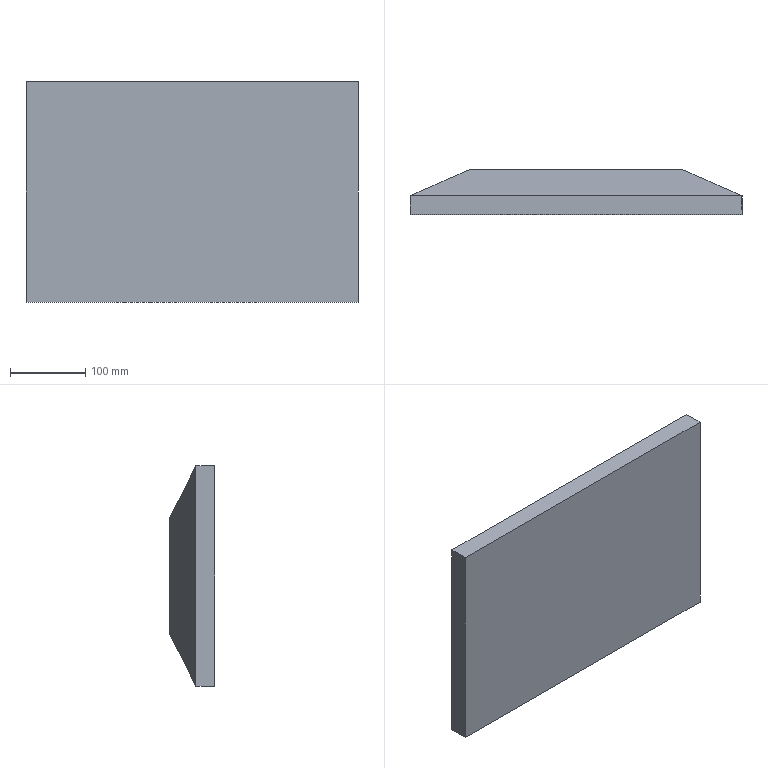Part | SolidWorks | features ICE 3, Extrusion 1 | 1 solid | 34 faces | box 440 x 60 x 292 mm | volume 6071392 mm3 | plane 18 | cylinder 16 | commonest cylinder face diameters 5 x16
STEP:
#1=CARTESIAN_POINT('',(182.5,40.,-186.));
#2=VERTEX_POINT('',#1);
#3=CARTESIAN_POINT('',(182.5,40.,-181.));
#4=VERTEX_POINT('',#3);
#5=CARTESIAN_POINT('',(182.5,40.,-183.5));
#6=DIRECTION('',(0.,1.,0.));
#7=DIRECTION('',(0.,0.,1.));
#8=AXIS2_PLACEMENT_3D('',#5,#6,#7);
#9=CIRCLE('',#8,2.5);
#10=EDGE_CURVE('',#2,#4,#9,.T.);
#11=ORIENTED_EDGE('',*,*,#10,.F.);
#12=CARTESIAN_POINT('',(182.5,60.,-186.));
#13=VERTEX_POINT('',#12);
#14=CARTESIAN_POINT('',(182.5,40.,-186.));
#15=DIRECTION('',(0.,1.,0.));
#16=VECTOR('',#15,1000.);
#17=LINE('',#14,#16);
#18=EDGE_CURVE('',#2,#13,#17,.T.);
#19=ORIENTED_EDGE('',*,*,#18,.T.);
#20=CARTESIAN_POINT('',(182.5,60.,-181.));
#21=VERTEX_POINT('',#20);
#22=CARTESIAN_POINT('',(182.5,60.,-183.5));
#23=DIRECTION('',(0.,1.,0.));
#24=DIRECTION('',(0.,0.,1.));
#25=AXIS2_PLACEMENT_3D('',#22,#23,#24);
#26=CIRCLE('',#25,2.5);
#27=EDGE_CURVE('',#13,#21,#26,.T.);
#28=ORIENTED_EDGE('',*,*,#27,.T.);
#29=CARTESIAN_POINT('',(182.5,40.,-181.));
#30=DIRECTION('',(0.,1.,0.));
#31=VECTOR('',#30,1000.);
#32=LINE('',#29,#31);
#33=EDGE_CURVE('',#4,#21,#32,.T.);
#34=ORIENTED_EDGE('',*,*,#33,.F.);
#35=EDGE_LOOP('',(#11,#19,#28,#34));
#36=FACE_OUTER_BOUND('',#35,.T.);
#37=CARTESIAN_POINT('',(182.5,40.,-183.5));
#38=DIRECTION('',(0.,1.,0.));
#39=DIRECTION('',(0.,0.,1.));
#40=AXIS2_PLACEMENT_3D('',#37,#38,#39);
#41=CYLINDRICAL_SURFACE('',#40,2.5);
#42=ADVANCED_FACE('',(#36),#41,.F.);
#43=CARTESIAN_POINT('',(170.,40.,-198.5));
#44=VERTEX_POINT('',#43);
#45=CARTESIAN_POINT('',(170.,40.,-193.5));
#46=VERTEX_POINT('',#45);
#47=CARTESIAN_POINT('',(170.,40.,-196.));
#48=DIRECTION('',(0.,1.,0.));
#49=DIRECTION('',(0.,0.,1.));
#50=AXIS2_PLACEMENT_3D('',#47,#48,#49);
#51=CIRCLE('',#50,2.5);
#52=EDGE_CURVE('',#44,#46,#51,.T.);
#53=ORIENTED_EDGE('',*,*,#52,.F.);
#54=CARTESIAN_POINT('',(170.,60.,-198.5));
#55=VERTEX_POINT('',#54);
#56=CARTESIAN_POINT('',(170.,40.,-198.5));
#57=DIRECTION('',(0.,1.,0.));
#58=VECTOR('',#57,1000.);
#59=LINE('',#56,#58);
#60=EDGE_CURVE('',#44,#55,#59,.T.);
#61=ORIENTED_EDGE('',*,*,#60,.T.);
#62=CARTESIAN_POINT('',(170.,60.,-193.5));
#63=VERTEX_POINT('',#62);
#64=CARTESIAN_POINT('',(170.,60.,-196.));
#65=DIRECTION('',(0.,1.,0.));
#66=DIRECTION('',(0.,0.,1.));
#67=AXIS2_PLACEMENT_3D('',#64,#65,#66);
#68=CIRCLE('',#67,2.5);
#69=EDGE_CURVE('',#55,#63,#68,.T.);
#70=ORIENTED_EDGE('',*,*,#69,.T.);
#71=CARTESIAN_POINT('',(170.,40.,-193.5));
#72=DIRECTION('',(0.,1.,0.));
#73=VECTOR('',#72,1000.);
#74=LINE('',#71,#73);
#75=EDGE_CURVE('',#46,#63,#74,.T.);
#76=ORIENTED_EDGE('',*,*,#75,.F.);
#77=EDGE_LOOP('',(#53,#61,#70,#76));
#78=FACE_OUTER_BOUND('',#77,.T.);
#79=CARTESIAN_POINT('',(170.,40.,-196.));
#80=DIRECTION('',(0.,1.,0.));
#81=DIRECTION('',(0.,0.,1.));
#82=AXIS2_PLACEMENT_3D('',#79,#80,#81);
#83=CYLINDRICAL_SURFACE('',#82,2.5);
#84=ADVANCED_FACE('',(#78),#83,.F.);
#85=CARTESIAN_POINT('',(182.5,40.,-111.));
#86=VERTEX_POINT('',#85);
#87=CARTESIAN_POINT('',(182.5,40.,-106.));
#88=VERTEX_POINT('',#87);
#89=CARTESIAN_POINT('',(182.5,40.,-108.5));
#90=DIRECTION('',(0.,1.,0.));
#91=DIRECTION('',(0.,0.,1.));
#92=AXIS2_PLACEMENT_3D('',#89,#90,#91);
#93=CIRCLE('',#92,2.5);
#94=EDGE_CURVE('',#86,#88,#93,.T.);
#95=ORIENTED_EDGE('',*,*,#94,.F.);
#96=CARTESIAN_POINT('',(182.5,60.,-111.));
#97=VERTEX_POINT('',#96);
#98=CARTESIAN_POINT('',(182.5,40.,-111.));
#99=DIRECTION('',(0.,1.,0.));
#100=VECTOR('',#99,1000.);
#101=LINE('',#98,#100);
#102=EDGE_CURVE('',#86,#97,#101,.T.);
#103=ORIENTED_EDGE('',*,*,#102,.T.);
#104=CARTESIAN_POINT('',(182.5,60.,-106.));
#105=VERTEX_POINT('',#104);
#106=CARTESIAN_POINT('',(182.5,60.,-108.5));
#107=DIRECTION('',(0.,1.,0.));
#108=DIRECTION('',(0.,0.,1.));
#109=AXIS2_PLACEMENT_3D('',#106,#107,#108);
#110=CIRCLE('',#109,2.5);
#111=EDGE_CURVE('',#97,#105,#110,.T.);
#112=ORIENTED_EDGE('',*,*,#111,.T.);
#113=CARTESIAN_POINT('',(182.5,40.,-106.));
#114=DIRECTION('',(0.,1.,0.));
#115=VECTOR('',#114,1000.);
#116=LINE('',#113,#115);
#117=EDGE_CURVE('',#88,#105,#116,.T.);
#118=ORIENTED_EDGE('',*,*,#117,.F.);
#119=EDGE_LOOP('',(#95,#103,#112,#118));
#120=FACE_OUTER_BOUND('',#119,.T.);
#121=CARTESIAN_POINT('',(182.5,40.,-108.5));
#122=DIRECTION('',(0.,1.,0.));
#123=DIRECTION('',(0.,0.,1.));
#124=AXIS2_PLACEMENT_3D('',#121,#122,#123);
#125=CYLINDRICAL_SURFACE('',#124,2.5);
#126=ADVANCED_FACE('',(#120),#125,.F.);
#127=CARTESIAN_POINT('',(170.,40.,-98.5));
#128=VERTEX_POINT('',#127);
#129=CARTESIAN_POINT('',(170.,40.,-93.5));
#130=VERTEX_POINT('',#129);
#131=CARTESIAN_POINT('',(170.,40.,-96.));
#132=DIRECTION('',(0.,1.,0.));
#133=DIRECTION('',(0.,0.,1.));
#134=AXIS2_PLACEMENT_3D('',#131,#132,#133);
#135=CIRCLE('',#134,2.5);
#136=EDGE_CURVE('',#128,#130,#135,.T.);
#137=ORIENTED_EDGE('',*,*,#136,.F.);
#138=CARTESIAN_POINT('',(170.,60.,-98.5));
#139=VERTEX_POINT('',#138);
#140=CARTESIAN_POINT('',(170.,40.,-98.5));
#141=DIRECTION('',(0.,1.,0.));
#142=VECTOR('',#141,1000.);
#143=LINE('',#140,#142);
#144=EDGE_CURVE('',#128,#139,#143,.T.);
#145=ORIENTED_EDGE('',*,*,#144,.T.);
#146=CARTESIAN_POINT('',(170.,60.,-93.5));
#147=VERTEX_POINT('',#146);
#148=CARTESIAN_POINT('',(170.,60.,-96.));
#149=DIRECTION('',(0.,1.,0.));
#150=DIRECTION('',(0.,0.,1.));
#151=AXIS2_PLACEMENT_3D('',#148,#149,#150);
#152=CIRCLE('',#151,2.5);
#153=EDGE_CURVE('',#139,#147,#152,.T.);
#154=ORIENTED_EDGE('',*,*,#153,.T.);
#155=CARTESIAN_POINT('',(170.,40.,-93.5));
#156=DIRECTION('',(0.,1.,0.));
#157=VECTOR('',#156,1000.);
#158=LINE('',#155,#157);
#159=EDGE_CURVE('',#130,#147,#158,.T.);
#160=ORIENTED_EDGE('',*,*,#159,.F.);
#161=EDGE_LOOP('',(#137,#145,#154,#160));
#162=FACE_OUTER_BOUND('',#161,.T.);
#163=CARTESIAN_POINT('',(170.,40.,-96.));
#164=DIRECTION('',(0.,1.,0.));
#165=DIRECTION('',(0.,0.,1.));
#166=AXIS2_PLACEMENT_3D('',#163,#164,#165);
#167=CYLINDRICAL_SURFACE('',#166,2.5);
#168=ADVANCED_FACE('',(#162),#167,.F.);
#169=CARTESIAN_POINT('',(257.5,40.,-111.));
#170=VERTEX_POINT('',#169);
#171=CARTESIAN_POINT('',(257.5,40.,-106.));
#172=VERTEX_POINT('',#171);
#173=CARTESIAN_POINT('',(257.5,40.,-108.5));
#174=DIRECTION('',(0.,1.,0.));
#175=DIRECTION('',(0.,0.,1.));
#176=AXIS2_PLACEMENT_3D('',#173,#174,#175);
#177=CIRCLE('',#176,2.5);
#178=EDGE_CURVE('',#170,#172,#177,.T.);
#179=ORIENTED_EDGE('',*,*,#178,.F.);
#180=CARTESIAN_POINT('',(257.5,60.,-111.));
#181=VERTEX_POINT('',#180);
#182=CARTESIAN_POINT('',(257.5,40.,-111.));
#183=DIRECTION('',(0.,1.,0.));
#184=VECTOR('',#183,1000.);
#185=LINE('',#182,#184);
#186=EDGE_CURVE('',#170,#181,#185,.T.);
#187=ORIENTED_EDGE('',*,*,#186,.T.);
#188=CARTESIAN_POINT('',(257.5,60.,-106.));
#189=VERTEX_POINT('',#188);
#190=CARTESIAN_POINT('',(257.5,60.,-108.5));
#191=DIRECTION('',(0.,1.,0.));
#192=DIRECTION('',(0.,0.,1.));
#193=AXIS2_PLACEMENT_3D('',#190,#191,#192);
#194=CIRCLE('',#193,2.5);
#195=EDGE_CURVE('',#181,#189,#194,.T.);
#196=ORIENTED_EDGE('',*,*,#195,.T.);
#197=CARTESIAN_POINT('',(257.5,40.,-106.));
#198=DIRECTION('',(0.,1.,0.));
#199=VECTOR('',#198,1000.);
#200=LINE('',#197,#199);
#201=EDGE_CURVE('',#172,#189,#200,.T.);
#202=ORIENTED_EDGE('',*,*,#201,.F.);
#203=EDGE_LOOP('',(#179,#187,#196,#202));
#204=FACE_OUTER_BOUND('',#203,.T.);
#205=CARTESIAN_POINT('',(257.5,40.,-108.5));
#206=DIRECTION('',(0.,1.,0.));
#207=DIRECTION('',(0.,0.,1.));
#208=AXIS2_PLACEMENT_3D('',#205,#206,#207);
#209=CYLINDRICAL_SURFACE('',#208,2.5);
#210=ADVANCED_FACE('',(#204),#209,.F.);
#211=CARTESIAN_POINT('',(270.,40.,-98.5));
#212=VERTEX_POINT('',#211);
#213=CARTESIAN_POINT('',(270.,40.,-93.5));
#214=VERTEX_POINT('',#213);
#215=CARTESIAN_POINT('',(270.,40.,-96.));
#216=DIRECTION('',(0.,1.,0.));
#217=DIRECTION('',(0.,0.,1.));
#218=AXIS2_PLACEMENT_3D('',#215,#216,#217);
#219=CIRCLE('',#218,2.5);
#220=EDGE_CURVE('',#212,#214,#219,.T.);
#221=ORIENTED_EDGE('',*,*,#220,.F.);
#222=CARTESIAN_POINT('',(270.,60.,-98.5));
#223=VERTEX_POINT('',#222);
#224=CARTESIAN_POINT('',(270.,40.,-98.5));
#225=DIRECTION('',(0.,1.,0.));
#226=VECTOR('',#225,1000.);
#227=LINE('',#224,#226);
#228=EDGE_CURVE('',#212,#223,#227,.T.);
#229=ORIENTED_EDGE('',*,*,#228,.T.);
#230=CARTESIAN_POINT('',(270.,60.,-93.5));
#231=VERTEX_POINT('',#230);
#232=CARTESIAN_POINT('',(270.,60.,-96.));
#233=DIRECTION('',(0.,1.,0.));
#234=DIRECTION('',(0.,0.,1.));
#235=AXIS2_PLACEMENT_3D('',#232,#233,#234);
#236=CIRCLE('',#235,2.5);
#237=EDGE_CURVE('',#223,#231,#236,.T.);
#238=ORIENTED_EDGE('',*,*,#237,.T.);
#239=CARTESIAN_POINT('',(270.,40.,-93.5));
#240=DIRECTION('',(0.,1.,0.));
#241=VECTOR('',#240,1000.);
#242=LINE('',#239,#241);
#243=EDGE_CURVE('',#214,#231,#242,.T.);
#244=ORIENTED_EDGE('',*,*,#243,.F.);
#245=EDGE_LOOP('',(#221,#229,#238,#244));
#246=FACE_OUTER_BOUND('',#245,.T.);
#247=CARTESIAN_POINT('',(270.,40.,-96.));
#248=DIRECTION('',(0.,1.,0.));
#249=DIRECTION('',(0.,0.,1.));
#250=AXIS2_PLACEMENT_3D('',#247,#248,#249);
#251=CYLINDRICAL_SURFACE('',#250,2.5);
#252=ADVANCED_FACE('',(#246),#251,.F.);
#253=CARTESIAN_POINT('',(257.5,40.,-186.));
#254=VERTEX_POINT('',#253);
#255=CARTESIAN_POINT('',(257.5,40.,-181.));
#256=VERTEX_POINT('',#255);
#257=CARTESIAN_POINT('',(257.5,40.,-183.5));
#258=DIRECTION('',(0.,1.,0.));
#259=DIRECTION('',(0.,0.,1.));
#260=AXIS2_PLACEMENT_3D('',#257,#258,#259);
#261=CIRCLE('',#260,2.5);
#262=EDGE_CURVE('',#254,#256,#261,.T.);
#263=ORIENTED_EDGE('',*,*,#262,.F.);
#264=CARTESIAN_POINT('',(257.5,60.,-186.));
#265=VERTEX_POINT('',#264);
#266=CARTESIAN_POINT('',(257.5,40.,-186.));
#267=DIRECTION('',(0.,1.,0.));
#268=VECTOR('',#267,1000.);
#269=LINE('',#266,#268);
#270=EDGE_CURVE('',#254,#265,#269,.T.);
#271=ORIENTED_EDGE('',*,*,#270,.T.);
#272=CARTESIAN_POINT('',(257.5,60.,-181.));
#273=VERTEX_POINT('',#272);
#274=CARTESIAN_POINT('',(257.5,60.,-183.5));
#275=DIRECTION('',(0.,1.,0.));
#276=DIRECTION('',(0.,0.,1.));
#277=AXIS2_PLACEMENT_3D('',#274,#275,#276);
#278=CIRCLE('',#277,2.5);
#279=EDGE_CURVE('',#265,#273,#278,.T.);
#280=ORIENTED_EDGE('',*,*,#279,.T.);
#281=CARTESIAN_POINT('',(257.5,40.,-181.));
#282=DIRECTION('',(0.,1.,0.));
#283=VECTOR('',#282,1000.);
#284=LINE('',#281,#283);
#285=EDGE_CURVE('',#256,#273,#284,.T.);
#286=ORIENTED_EDGE('',*,*,#285,.F.);
#287=EDGE_LOOP('',(#263,#271,#280,#286));
#288=FACE_OUTER_BOUND('',#287,.T.);
#289=CARTESIAN_POINT('',(257.5,40.,-183.5));
#290=DIRECTION('',(0.,1.,0.));
#291=DIRECTION('',(0.,0.,1.));
#292=AXIS2_PLACEMENT_3D('',#289,#290,#291);
#293=CYLINDRICAL_SURFACE('',#292,2.5);
#294=ADVANCED_FACE('',(#288),#293,.F.);
#295=CARTESIAN_POINT('',(270.,40.,-198.5));
#296=VERTEX_POINT('',#295);
#297=CARTESIAN_POINT('',(270.,40.,-193.5));
#298=VERTEX_POINT('',#297);
#299=CARTESIAN_POINT('',(270.,40.,-196.));
#300=DIRECTION('',(0.,1.,0.));
#301=DIRECTION('',(0.,0.,1.));
#302=AXIS2_PLACEMENT_3D('',#299,#300,#301);
#303=CIRCLE('',#302,2.5);
#304=EDGE_CURVE('',#296,#298,#303,.T.);
#305=ORIENTED_EDGE('',*,*,#304,.F.);
#306=CARTESIAN_POINT('',(270.,60.,-198.5));
#307=VERTEX_POINT('',#306);
#308=CARTESIAN_POINT('',(270.,40.,-198.5));
#309=DIRECTION('',(0.,1.,0.));
#310=VECTOR('',#309,1000.);
#311=LINE('',#308,#310);
#312=EDGE_CURVE('',#296,#307,#311,.T.);
#313=ORIENTED_EDGE('',*,*,#312,.T.);
#314=CARTESIAN_POINT('',(270.,60.,-193.5));
#315=VERTEX_POINT('',#314);
#316=CARTESIAN_POINT('',(270.,60.,-196.));
#317=DIRECTION('',(0.,1.,0.));
#318=DIRECTION('',(0.,0.,1.));
#319=AXIS2_PLACEMENT_3D('',#316,#317,#318);
#320=CIRCLE('',#319,2.5);
#321=EDGE_CURVE('',#307,#315,#320,.T.);
#322=ORIENTED_EDGE('',*,*,#321,.T.);
#323=CARTESIAN_POINT('',(270.,40.,-193.5));
#324=DIRECTION('',(0.,1.,0.));
#325=VECTOR('',#324,1000.);
#326=LINE('',#323,#325);
#327=EDGE_CURVE('',#298,#315,#326,.T.);
#328=ORIENTED_EDGE('',*,*,#327,.F.);
#329=EDGE_LOOP('',(#305,#313,#322,#328));
#330=FACE_OUTER_BOUND('',#329,.T.);
#331=CARTESIAN_POINT('',(270.,40.,-196.));
#332=DIRECTION('',(0.,1.,0.));
#333=DIRECTION('',(0.,0.,1.));
#334=AXIS2_PLACEMENT_3D('',#331,#332,#333);
#335=CYLINDRICAL_SURFACE('',#334,2.5);
#336=ADVANCED_FACE('',(#330),#335,.F.);
#337=CARTESIAN_POINT('',(0.,25.,0.));
#338=VERTEX_POINT('',#337);
#339=CARTESIAN_POINT('',(0.,0.,0.));
#340=VERTEX_POINT('',#339);
#341=CARTESIAN_POINT('',(0.,60.,0.));
#342=DIRECTION('',(0.,-1.,0.));
#343=VECTOR('',#342,1000.);
#344=LINE('',#341,#343);
#345=EDGE_CURVE('',#338,#340,#344,.T.);
#346=ORIENTED_EDGE('',*,*,#345,.F.);
#347=CARTESIAN_POINT('',(0.,25.,-292.));
#348=VERTEX_POINT('',#347);
#349=CARTESIAN_POINT('',(0.,25.,87.));
#350=DIRECTION('',(0.,0.,-1.));
#351=VECTOR('',#350,1000.);
#352=LINE('',#349,#351);
#353=EDGE_CURVE('',#338,#348,#352,.T.);
#354=ORIENTED_EDGE('',*,*,#353,.T.);
#355=CARTESIAN_POINT('',(0.,0.,-292.));
#356=VERTEX_POINT('',#355);
#357=CARTESIAN_POINT('',(0.,60.,-292.));
#358=DIRECTION('',(0.,-1.,0.));
#359=VECTOR('',#358,1000.);
#360=LINE('',#357,#359);
#361=EDGE_CURVE('',#348,#356,#360,.T.);
#362=ORIENTED_EDGE('',*,*,#361,.T.);
#363=CARTESIAN_POINT('',(0.,0.,0.));
#364=DIRECTION('',(0.,0.,1.));
#365=VECTOR('',#364,1000.);
#366=LINE('',#363,#365);
#367=EDGE_CURVE('',#356,#340,#366,.T.);
#368=ORIENTED_EDGE('',*,*,#367,.T.);
#369=EDGE_LOOP('',(#346,#354,#362,#368));
#370=FACE_OUTER_BOUND('',#369,.T.);
#371=CARTESIAN_POINT('',(0.,60.,0.));
#372=DIRECTION('',(1.,0.,0.));
#373=DIRECTION('',(0.,0.,-1.));
#374=AXIS2_PLACEMENT_3D('',#371,#372,#373);
#375=PLANE('',#374);
#376=ADVANCED_FACE('',(#370),#375,.F.);
#377=CARTESIAN_POINT('',(440.,25.,0.));
#378=VERTEX_POINT('',#377);
#379=CARTESIAN_POINT('',(440.,0.,0.));
#380=VERTEX_POINT('',#379);
#381=CARTESIAN_POINT('',(440.,60.,0.));
#382=DIRECTION('',(0.,-1.,0.));
#383=VECTOR('',#382,1000.);
#384=LINE('',#381,#383);
#385=EDGE_CURVE('',#378,#380,#384,.T.);
#386=ORIENTED_EDGE('',*,*,#385,.F.);
#387=CARTESIAN_POINT('',(467.,25.,0.));
#388=DIRECTION('',(-1.,0.,0.));
#389=VECTOR('',#388,1000.);
#390=LINE('',#387,#389);
#391=EDGE_CURVE('',#378,#338,#390,.T.);
#392=ORIENTED_EDGE('',*,*,#391,.T.);
#393=ORIENTED_EDGE('',*,*,#345,.T.);
#394=CARTESIAN_POINT('',(0.,0.,0.));
#395=DIRECTION('',(1.,0.,0.));
#396=VECTOR('',#395,1000.);
#397=LINE('',#394,#396);
#398=EDGE_CURVE('',#340,#380,#397,.T.);
#399=ORIENTED_EDGE('',*,*,#398,.T.);
#400=EDGE_LOOP('',(#386,#392,#393,#399));
#401=FACE_OUTER_BOUND('',#400,.T.);
#402=CARTESIAN_POINT('',(0.,60.,0.));
#403=DIRECTION('',(0.,0.,-1.));
#404=DIRECTION('',(-1.,0.,0.));
#405=AXIS2_PLACEMENT_3D('',#402,#403,#404);
#406=PLANE('',#405);
#407=ADVANCED_FACE('',(#401),#406,.F.);
#408=CARTESIAN_POINT('',(440.,25.,-292.));
#409=VERTEX_POINT('',#408);
#410=CARTESIAN_POINT('',(440.,0.,-292.));
#411=VERTEX_POINT('',#410);
#412=CARTESIAN_POINT('',(440.,60.,-292.));
#413=DIRECTION('',(0.,-1.,0.));
#414=VECTOR('',#413,1000.);
#415=LINE('',#412,#414);
#416=EDGE_CURVE('',#409,#411,#415,.T.);
#417=ORIENTED_EDGE('',*,*,#416,.F.);
#418=CARTESIAN_POINT('',(440.,25.,87.));
#419=DIRECTION('',(0.,0.,-1.));
#420=VECTOR('',#419,1000.);
#421=LINE('',#418,#420);
#422=EDGE_CURVE('',#378,#409,#421,.T.);
#423=ORIENTED_EDGE('',*,*,#422,.F.);
#424=ORIENTED_EDGE('',*,*,#385,.T.);
#425=CARTESIAN_POINT('',(440.,0.,0.));
#426=DIRECTION('',(0.,0.,-1.));
#427=VECTOR('',#426,1000.);
#428=LINE('',#425,#427);
#429=EDGE_CURVE('',#380,#411,#428,.T.);
#430=ORIENTED_EDGE('',*,*,#429,.T.);
#431=EDGE_LOOP('',(#417,#423,#424,#430));
#432=FACE_OUTER_BOUND('',#431,.T.);
#433=CARTESIAN_POINT('',(440.,60.,0.));
#434=DIRECTION('',(-1.,0.,0.));
#435=DIRECTION('',(0.,0.,1.));
#436=AXIS2_PLACEMENT_3D('',#433,#434,#435);
#437=PLANE('',#436);
#438=ADVANCED_FACE('',(#432),#437,.F.);
#439=ORIENTED_EDGE('',*,*,#361,.F.);
#440=CARTESIAN_POINT('',(467.,25.,-292.));
#441=DIRECTION('',(-1.,0.,0.));
#442=VECTOR('',#441,1000.);
#443=LINE('',#440,#442);
#444=EDGE_CURVE('',#409,#348,#443,.T.);
#445=ORIENTED_EDGE('',*,*,#444,.F.);
#446=ORIENTED_EDGE('',*,*,#416,.T.);
#447=CARTESIAN_POINT('',(0.,0.,-292.));
#448=DIRECTION('',(-1.,0.,0.));
#449=VECTOR('',#448,1000.);
#450=LINE('',#447,#449);
#451=EDGE_CURVE('',#411,#356,#450,.T.);
#452=ORIENTED_EDGE('',*,*,#451,.T.);
#453=EDGE_LOOP('',(#439,#445,#446,#452));
#454=FACE_OUTER_BOUND('',#453,.T.);
#455=CARTESIAN_POINT('',(0.,60.,-292.));
#456=DIRECTION('',(0.,0.,1.));
#457=DIRECTION('',(1.,0.,0.));
#458=AXIS2_PLACEMENT_3D('',#455,#456,#457);
#459=PLANE('',#458);
#460=ADVANCED_FACE('',(#454),#459,.F.);
#461=CARTESIAN_POINT('',(182.5,60.,-183.5));
#462=DIRECTION('',(0.,1.,0.));
#463=DIRECTION('',(0.,0.,1.));
#464=AXIS2_PLACEMENT_3D('',#461,#462,#463);
#465=CIRCLE('',#464,2.5);
#466=EDGE_CURVE('',#21,#13,#465,.T.);
#467=ORIENTED_EDGE('',*,*,#466,.F.);
#468=ORIENTED_EDGE('',*,*,#27,.F.);
#469=EDGE_LOOP('',(#467,#468));
#470=FACE_BOUND('',#469,.T.);
#471=CARTESIAN_POINT('',(170.,60.,-196.));
#472=DIRECTION('',(0.,1.,0.));
#473=DIRECTION('',(0.,0.,1.));
#474=AXIS2_PLACEMENT_3D('',#471,#472,#473);
#475=CIRCLE('',#474,2.5);
#476=EDGE_CURVE('',#63,#55,#475,.T.);
#477=ORIENTED_EDGE('',*,*,#476,.F.);
#478=ORIENTED_EDGE('',*,*,#69,.F.);
#479=EDGE_LOOP('',(#477,#478));
#480=FACE_BOUND('',#479,.T.);
#481=CARTESIAN_POINT('',(182.5,60.,-108.5));
#482=DIRECTION('',(0.,1.,0.));
#483=DIRECTION('',(0.,0.,1.));
#484=AXIS2_PLACEMENT_3D('',#481,#482,#483);
#485=CIRCLE('',#484,2.5);
#486=EDGE_CURVE('',#105,#97,#485,.T.);
#487=ORIENTED_EDGE('',*,*,#486,.F.);
#488=ORIENTED_EDGE('',*,*,#111,.F.);
#489=EDGE_LOOP('',(#487,#488));
#490=FACE_BOUND('',#489,.T.);
#491=CARTESIAN_POINT('',(170.,60.,-96.));
#492=DIRECTION('',(0.,1.,0.));
#493=DIRECTION('',(0.,0.,1.));
#494=AXIS2_PLACEMENT_3D('',#491,#492,#493);
#495=CIRCLE('',#494,2.5);
#496=EDGE_CURVE('',#147,#139,#495,.T.);
#497=ORIENTED_EDGE('',*,*,#496,.F.);
#498=ORIENTED_EDGE('',*,*,#153,.F.);
#499=EDGE_LOOP('',(#497,#498));
#500=FACE_BOUND('',#499,.T.);
#501=CARTESIAN_POINT('',(257.5,60.,-108.5));
#502=DIRECTION('',(0.,1.,0.));
#503=DIRECTION('',(0.,0.,1.));
#504=AXIS2_PLACEMENT_3D('',#501,#502,#503);
#505=CIRCLE('',#504,2.5);
#506=EDGE_CURVE('',#189,#181,#505,.T.);
#507=ORIENTED_EDGE('',*,*,#506,.F.);
#508=ORIENTED_EDGE('',*,*,#195,.F.);
#509=EDGE_LOOP('',(#507,#508));
#510=FACE_BOUND('',#509,.T.);
#511=CARTESIAN_POINT('',(270.,60.,-96.));
#512=DIRECTION('',(0.,1.,0.));
#513=DIRECTION('',(0.,0.,1.));
#514=AXIS2_PLACEMENT_3D('',#511,#512,#513);
#515=CIRCLE('',#514,2.5);
#516=EDGE_CURVE('',#231,#223,#515,.T.);
#517=ORIENTED_EDGE('',*,*,#516,.F.);
#518=ORIENTED_EDGE('',*,*,#237,.F.);
#519=EDGE_LOOP('',(#517,#518));
#520=FACE_BOUND('',#519,.T.);
#521=CARTESIAN_POINT('',(257.5,60.,-183.5));
#522=DIRECTION('',(0.,1.,0.));
#523=DIRECTION('',(0.,0.,1.));
#524=AXIS2_PLACEMENT_3D('',#521,#522,#523);
#525=CIRCLE('',#524,2.5);
#526=EDGE_CURVE('',#273,#265,#525,.T.);
#527=ORIENTED_EDGE('',*,*,#526,.F.);
#528=ORIENTED_EDGE('',*,*,#279,.F.);
#529=EDGE_LOOP('',(#527,#528));
#530=FACE_BOUND('',#529,.T.);
#531=CARTESIAN_POINT('',(270.,60.,-196.));
#532=DIRECTION('',(0.,1.,0.));
#533=DIRECTION('',(0.,0.,1.));
#534=AXIS2_PLACEMENT_3D('',#531,#532,#533);
#535=CIRCLE('',#534,2.5);
#536=EDGE_CURVE('',#315,#307,#535,.T.);
#537=ORIENTED_EDGE('',*,*,#536,.F.);
#538=ORIENTED_EDGE('',*,*,#321,.F.);
#539=EDGE_LOOP('',(#537,#538));
#540=FACE_BOUND('',#539,.T.);
#541=CARTESIAN_POINT('',(80.,60.,-222.));
#542=VERTEX_POINT('',#541);
#543=CARTESIAN_POINT('',(80.,60.,-70.));
#544=VERTEX_POINT('',#543);
#545=CARTESIAN_POINT('',(80.,60.,-292.));
#546=DIRECTION('',(0.,0.,1.));
#547=VECTOR('',#546,1000.);
#548=LINE('',#545,#547);
#549=EDGE_CURVE('',#542,#544,#548,.T.);
#550=ORIENTED_EDGE('',*,*,#549,.T.);
#551=CARTESIAN_POINT('',(360.,60.,-70.));
#552=VERTEX_POINT('',#551);
#553=CARTESIAN_POINT('',(467.,60.,-70.));
#554=DIRECTION('',(-1.,0.,0.));
#555=VECTOR('',#554,1000.);
#556=LINE('',#553,#555);
#557=EDGE_CURVE('',#552,#544,#556,.T.);
#558=ORIENTED_EDGE('',*,*,#557,.F.);
#559=CARTESIAN_POINT('',(360.,60.,-222.));
#560=VERTEX_POINT('',#559);
#561=CARTESIAN_POINT('',(360.,60.,-292.));
#562=DIRECTION('',(0.,0.,-1.));
#563=VECTOR('',#562,1000.);
#564=LINE('',#561,#563);
#565=EDGE_CURVE('',#552,#560,#564,.T.);
#566=ORIENTED_EDGE('',*,*,#565,.T.);
#567=CARTESIAN_POINT('',(467.,60.,-222.));
#568=DIRECTION('',(-1.,0.,0.));
#569=VECTOR('',#568,1000.);
#570=LINE('',#567,#569);
#571=EDGE_CURVE('',#560,#542,#570,.T.);
#572=ORIENTED_EDGE('',*,*,#571,.T.);
#573=EDGE_LOOP('',(#550,#558,#566,#572));
#574=FACE_OUTER_BOUND('',#573,.T.);
#575=CARTESIAN_POINT('',(0.,60.,-292.));
#576=DIRECTION('',(0.,-1.,0.));
#577=DIRECTION('',(0.,0.,-1.));
#578=AXIS2_PLACEMENT_3D('',#575,#576,#577);
#579=PLANE('',#578);
#580=ADVANCED_FACE('',(#470,#480,#490,#500,#510,#520,#530,#540,#574),#579,.F.);
#581=ORIENTED_EDGE('',*,*,#367,.F.);
#582=ORIENTED_EDGE('',*,*,#451,.F.);
#583=ORIENTED_EDGE('',*,*,#429,.F.);
#584=ORIENTED_EDGE('',*,*,#398,.F.);
#585=EDGE_LOOP('',(#581,#582,#583,#584));
#586=FACE_OUTER_BOUND('',#585,.T.);
#587=CARTESIAN_POINT('',(0.,0.,-292.));
#588=DIRECTION('',(0.,-1.,0.));
#589=DIRECTION('',(0.,0.,-1.));
#590=AXIS2_PLACEMENT_3D('',#587,#588,#589);
#591=PLANE('',#590);
#592=ADVANCED_FACE('',(#586),#591,.T.);
#593=ORIENTED_EDGE('',*,*,#565,.F.);
#594=CARTESIAN_POINT('',(430.196,29.289,-8.579));
#595=DIRECTION('',(0.7148,-0.3127,0.6255));
#596=VECTOR('',#595,1000.);
#597=LINE('',#594,#596);
#598=EDGE_CURVE('',#552,#378,#597,.T.);
#599=ORIENTED_EDGE('',*,*,#598,.T.);
#600=ORIENTED_EDGE('',*,*,#422,.T.);
#601=CARTESIAN_POINT('',(221.844,120.443,-101.114));
#602=DIRECTION('',(-0.7148,0.3127,0.6255));
#603=VECTOR('',#602,1000.);
#604=LINE('',#601,#603);
#605=EDGE_CURVE('',#409,#560,#604,.T.);
#606=ORIENTED_EDGE('',*,*,#605,.T.);
#607=EDGE_LOOP('',(#593,#599,#600,#606));
#608=FACE_OUTER_BOUND('',#607,.T.);
#609=CARTESIAN_POINT('',(360.,60.,87.));
#610=DIRECTION('',(-0.4008,-0.9162,0.));
#611=DIRECTION('',(0.9162,-0.4008,0.));
#612=AXIS2_PLACEMENT_3D('',#609,#610,#611);
#613=PLANE('',#612);
#614=ADVANCED_FACE('',(#608),#613,.F.);
#615=ORIENTED_EDGE('',*,*,#353,.F.);
#616=CARTESIAN_POINT('',(9.804,29.289,-8.579));
#617=DIRECTION('',(0.7148,0.3127,-0.6255));
#618=VECTOR('',#617,1000.);
#619=LINE('',#616,#618);
#620=EDGE_CURVE('',#338,#544,#619,.T.);
#621=ORIENTED_EDGE('',*,*,#620,.T.);
#622=ORIENTED_EDGE('',*,*,#549,.F.);
#623=CARTESIAN_POINT('',(218.156,120.443,-101.114));
#624=DIRECTION('',(-0.7148,-0.3127,-0.6255));
#625=VECTOR('',#624,1000.);
#626=LINE('',#623,#625);
#627=EDGE_CURVE('',#542,#348,#626,.T.);
#628=ORIENTED_EDGE('',*,*,#627,.T.);
#629=EDGE_LOOP('',(#615,#621,#622,#628));
#630=FACE_OUTER_BOUND('',#629,.T.);
#631=CARTESIAN_POINT('',(80.,60.,87.));
#632=DIRECTION('',(0.4008,-0.9162,0.));
#633=DIRECTION('',(0.9162,0.4008,0.));
#634=AXIS2_PLACEMENT_3D('',#631,#632,#633);
#635=PLANE('',#634);
#636=ADVANCED_FACE('',(#630),#635,.F.);
#637=ORIENTED_EDGE('',*,*,#444,.T.);
#638=ORIENTED_EDGE('',*,*,#627,.F.);
#639=ORIENTED_EDGE('',*,*,#571,.F.);
#640=ORIENTED_EDGE('',*,*,#605,.F.);
#641=EDGE_LOOP('',(#637,#638,#639,#640));
#642=FACE_OUTER_BOUND('',#641,.T.);
#643=CARTESIAN_POINT('',(467.,60.,-222.));
#644=DIRECTION('',(0.,-0.8944,0.4472));
#645=DIRECTION('',(0.,-0.4472,-0.8944));
#646=AXIS2_PLACEMENT_3D('',#643,#644,#645);
#647=PLANE('',#646);
#648=ADVANCED_FACE('',(#642),#647,.F.);
#649=ORIENTED_EDGE('',*,*,#557,.T.);
#650=ORIENTED_EDGE('',*,*,#620,.F.);
#651=ORIENTED_EDGE('',*,*,#391,.F.);
#652=ORIENTED_EDGE('',*,*,#598,.F.);
#653=EDGE_LOOP('',(#649,#650,#651,#652));
#654=FACE_OUTER_BOUND('',#653,.T.);
#655=CARTESIAN_POINT('',(467.,60.,-70.));
#656=DIRECTION('',(0.,-0.8944,-0.4472));
#657=DIRECTION('',(0.,0.4472,-0.8944));
#658=AXIS2_PLACEMENT_3D('',#655,#656,#657);
#659=PLANE('',#658);
#660=ADVANCED_FACE('',(#654),#659,.F.);
#661=ORIENTED_EDGE('',*,*,#312,.F.);
#662=CARTESIAN_POINT('',(270.,40.,-196.));
#663=DIRECTION('',(0.,1.,0.));
#664=DIRECTION('',(0.,0.,1.));
#665=AXIS2_PLACEMENT_3D('',#662,#663,#664);
#666=CIRCLE('',#665,2.5);
#667=EDGE_CURVE('',#298,#296,#666,.T.);
#668=ORIENTED_EDGE('',*,*,#667,.F.);
#669=ORIENTED_EDGE('',*,*,#327,.T.);
#670=ORIENTED_EDGE('',*,*,#536,.T.);
#671=EDGE_LOOP('',(#661,#668,#669,#670));
#672=FACE_OUTER_BOUND('',#671,.T.);
#673=CARTESIAN_POINT('',(270.,40.,-196.));
#674=DIRECTION('',(0.,1.,0.));
#675=DIRECTION('',(0.,0.,1.));
#676=AXIS2_PLACEMENT_3D('',#673,#674,#675);
#677=CYLINDRICAL_SURFACE('',#676,2.5);
#678=ADVANCED_FACE('',(#672),#677,.F.);
#679=ORIENTED_EDGE('',*,*,#667,.T.);
#680=ORIENTED_EDGE('',*,*,#304,.T.);
#681=EDGE_LOOP('',(#679,#680));
#682=FACE_OUTER_BOUND('',#681,.T.);
#683=CARTESIAN_POINT('',(270.,40.,-196.));
#684=DIRECTION('',(0.,1.,0.));
#685=DIRECTION('',(0.,0.,1.));
#686=AXIS2_PLACEMENT_3D('',#683,#684,#685);
#687=PLANE('',#686);
#688=ADVANCED_FACE('',(#682),#687,.T.);
#689=ORIENTED_EDGE('',*,*,#270,.F.);
#690=CARTESIAN_POINT('',(257.5,40.,-183.5));
#691=DIRECTION('',(0.,1.,0.));
#692=DIRECTION('',(0.,0.,1.));
#693=AXIS2_PLACEMENT_3D('',#690,#691,#692);
#694=CIRCLE('',#693,2.5);
#695=EDGE_CURVE('',#256,#254,#694,.T.);
#696=ORIENTED_EDGE('',*,*,#695,.F.);
#697=ORIENTED_EDGE('',*,*,#285,.T.);
#698=ORIENTED_EDGE('',*,*,#526,.T.);
#699=EDGE_LOOP('',(#689,#696,#697,#698));
#700=FACE_OUTER_BOUND('',#699,.T.);
#701=CARTESIAN_POINT('',(257.5,40.,-183.5));
#702=DIRECTION('',(0.,1.,0.));
#703=DIRECTION('',(0.,0.,1.));
#704=AXIS2_PLACEMENT_3D('',#701,#702,#703);
#705=CYLINDRICAL_SURFACE('',#704,2.5);
#706=ADVANCED_FACE('',(#700),#705,.F.);
#707=ORIENTED_EDGE('',*,*,#695,.T.);
#708=ORIENTED_EDGE('',*,*,#262,.T.);
#709=EDGE_LOOP('',(#707,#708));
#710=FACE_OUTER_BOUND('',#709,.T.);
#711=CARTESIAN_POINT('',(257.5,40.,-183.5));
#712=DIRECTION('',(0.,1.,0.));
#713=DIRECTION('',(0.,0.,1.));
#714=AXIS2_PLACEMENT_3D('',#711,#712,#713);
#715=PLANE('',#714);
#716=ADVANCED_FACE('',(#710),#715,.T.);
#717=ORIENTED_EDGE('',*,*,#228,.F.);
#718=CARTESIAN_POINT('',(270.,40.,-96.));
#719=DIRECTION('',(0.,1.,0.));
#720=DIRECTION('',(0.,0.,1.));
#721=AXIS2_PLACEMENT_3D('',#718,#719,#720);
#722=CIRCLE('',#721,2.5);
#723=EDGE_CURVE('',#214,#212,#722,.T.);
#724=ORIENTED_EDGE('',*,*,#723,.F.);
#725=ORIENTED_EDGE('',*,*,#243,.T.);
#726=ORIENTED_EDGE('',*,*,#516,.T.);
#727=EDGE_LOOP('',(#717,#724,#725,#726));
#728=FACE_OUTER_BOUND('',#727,.T.);
#729=CARTESIAN_POINT('',(270.,40.,-96.));
#730=DIRECTION('',(0.,1.,0.));
#731=DIRECTION('',(0.,0.,1.));
#732=AXIS2_PLACEMENT_3D('',#729,#730,#731);
#733=CYLINDRICAL_SURFACE('',#732,2.5);
#734=ADVANCED_FACE('',(#728),#733,.F.);
#735=ORIENTED_EDGE('',*,*,#723,.T.);
#736=ORIENTED_EDGE('',*,*,#220,.T.);
#737=EDGE_LOOP('',(#735,#736));
#738=FACE_OUTER_BOUND('',#737,.T.);
#739=CARTESIAN_POINT('',(270.,40.,-96.));
#740=DIRECTION('',(0.,1.,0.));
#741=DIRECTION('',(0.,0.,1.));
#742=AXIS2_PLACEMENT_3D('',#739,#740,#741);
#743=PLANE('',#742);
#744=ADVANCED_FACE('',(#738),#743,.T.);
#745=ORIENTED_EDGE('',*,*,#186,.F.);
#746=CARTESIAN_POINT('',(257.5,40.,-108.5));
#747=DIRECTION('',(0.,1.,0.));
#748=DIRECTION('',(0.,0.,1.));
#749=AXIS2_PLACEMENT_3D('',#746,#747,#748);
#750=CIRCLE('',#749,2.5);
#751=EDGE_CURVE('',#172,#170,#750,.T.);
#752=ORIENTED_EDGE('',*,*,#751,.F.);
#753=ORIENTED_EDGE('',*,*,#201,.T.);
#754=ORIENTED_EDGE('',*,*,#506,.T.);
#755=EDGE_LOOP('',(#745,#752,#753,#754));
#756=FACE_OUTER_BOUND('',#755,.T.);
#757=CARTESIAN_POINT('',(257.5,40.,-108.5));
#758=DIRECTION('',(0.,1.,0.));
#759=DIRECTION('',(0.,0.,1.));
#760=AXIS2_PLACEMENT_3D('',#757,#758,#759);
#761=CYLINDRICAL_SURFACE('',#760,2.5);
#762=ADVANCED_FACE('',(#756),#761,.F.);
#763=ORIENTED_EDGE('',*,*,#751,.T.);
#764=ORIENTED_EDGE('',*,*,#178,.T.);
#765=EDGE_LOOP('',(#763,#764));
#766=FACE_OUTER_BOUND('',#765,.T.);
#767=CARTESIAN_POINT('',(257.5,40.,-108.5));
#768=DIRECTION('',(0.,1.,0.));
#769=DIRECTION('',(0.,0.,1.));
#770=AXIS2_PLACEMENT_3D('',#767,#768,#769);
#771=PLANE('',#770);
#772=ADVANCED_FACE('',(#766),#771,.T.);
#773=ORIENTED_EDGE('',*,*,#144,.F.);
#774=CARTESIAN_POINT('',(170.,40.,-96.));
#775=DIRECTION('',(0.,1.,0.));
#776=DIRECTION('',(0.,0.,1.));
#777=AXIS2_PLACEMENT_3D('',#774,#775,#776);
#778=CIRCLE('',#777,2.5);
#779=EDGE_CURVE('',#130,#128,#778,.T.);
#780=ORIENTED_EDGE('',*,*,#779,.F.);
#781=ORIENTED_EDGE('',*,*,#159,.T.);
#782=ORIENTED_EDGE('',*,*,#496,.T.);
#783=EDGE_LOOP('',(#773,#780,#781,#782));
#784=FACE_OUTER_BOUND('',#783,.T.);
#785=CARTESIAN_POINT('',(170.,40.,-96.));
#786=DIRECTION('',(0.,1.,0.));
#787=DIRECTION('',(0.,0.,1.));
#788=AXIS2_PLACEMENT_3D('',#785,#786,#787);
#789=CYLINDRICAL_SURFACE('',#788,2.5);
#790=ADVANCED_FACE('',(#784),#789,.F.);
#791=ORIENTED_EDGE('',*,*,#779,.T.);
#792=ORIENTED_EDGE('',*,*,#136,.T.);
#793=EDGE_LOOP('',(#791,#792));
#794=FACE_OUTER_BOUND('',#793,.T.);
#795=CARTESIAN_POINT('',(170.,40.,-96.));
#796=DIRECTION('',(0.,1.,0.));
#797=DIRECTION('',(0.,0.,1.));
#798=AXIS2_PLACEMENT_3D('',#795,#796,#797);
#799=PLANE('',#798);
#800=ADVANCED_FACE('',(#794),#799,.T.);
#801=ORIENTED_EDGE('',*,*,#102,.F.);
#802=CARTESIAN_POINT('',(182.5,40.,-108.5));
#803=DIRECTION('',(0.,1.,0.));
#804=DIRECTION('',(0.,0.,1.));
#805=AXIS2_PLACEMENT_3D('',#802,#803,#804);
#806=CIRCLE('',#805,2.5);
#807=EDGE_CURVE('',#88,#86,#806,.T.);
#808=ORIENTED_EDGE('',*,*,#807,.F.);
#809=ORIENTED_EDGE('',*,*,#117,.T.);
#810=ORIENTED_EDGE('',*,*,#486,.T.);
#811=EDGE_LOOP('',(#801,#808,#809,#810));
#812=FACE_OUTER_BOUND('',#811,.T.);
#813=CARTESIAN_POINT('',(182.5,40.,-108.5));
#814=DIRECTION('',(0.,1.,0.));
#815=DIRECTION('',(0.,0.,1.));
#816=AXIS2_PLACEMENT_3D('',#813,#814,#815);
#817=CYLINDRICAL_SURFACE('',#816,2.5);
#818=ADVANCED_FACE('',(#812),#817,.F.);
#819=ORIENTED_EDGE('',*,*,#807,.T.);
#820=ORIENTED_EDGE('',*,*,#94,.T.);
#821=EDGE_LOOP('',(#819,#820));
#822=FACE_OUTER_BOUND('',#821,.T.);
#823=CARTESIAN_POINT('',(182.5,40.,-108.5));
#824=DIRECTION('',(0.,1.,0.));
#825=DIRECTION('',(0.,0.,1.));
#826=AXIS2_PLACEMENT_3D('',#823,#824,#825);
#827=PLANE('',#826);
#828=ADVANCED_FACE('',(#822),#827,.T.);
#829=ORIENTED_EDGE('',*,*,#60,.F.);
#830=CARTESIAN_POINT('',(170.,40.,-196.));
#831=DIRECTION('',(0.,1.,0.));
#832=DIRECTION('',(0.,0.,1.));
#833=AXIS2_PLACEMENT_3D('',#830,#831,#832);
#834=CIRCLE('',#833,2.5);
#835=EDGE_CURVE('',#46,#44,#834,.T.);
#836=ORIENTED_EDGE('',*,*,#835,.F.);
#837=ORIENTED_EDGE('',*,*,#75,.T.);
#838=ORIENTED_EDGE('',*,*,#476,.T.);
#839=EDGE_LOOP('',(#829,#836,#837,#838));
#840=FACE_OUTER_BOUND('',#839,.T.);
#841=CARTESIAN_POINT('',(170.,40.,-196.));
#842=DIRECTION('',(0.,1.,0.));
#843=DIRECTION('',(0.,0.,1.));
#844=AXIS2_PLACEMENT_3D('',#841,#842,#843);
#845=CYLINDRICAL_SURFACE('',#844,2.5);
#846=ADVANCED_FACE('',(#840),#845,.F.);
#847=ORIENTED_EDGE('',*,*,#835,.T.);
#848=ORIENTED_EDGE('',*,*,#52,.T.);
#849=EDGE_LOOP('',(#847,#848));
#850=FACE_OUTER_BOUND('',#849,.T.);
#851=CARTESIAN_POINT('',(170.,40.,-196.));
#852=DIRECTION('',(0.,1.,0.));
#853=DIRECTION('',(0.,0.,1.));
#854=AXIS2_PLACEMENT_3D('',#851,#852,#853);
#855=PLANE('',#854);
#856=ADVANCED_FACE('',(#850),#855,.T.);
#857=ORIENTED_EDGE('',*,*,#18,.F.);
#858=CARTESIAN_POINT('',(182.5,40.,-183.5));
#859=DIRECTION('',(0.,1.,0.));
#860=DIRECTION('',(0.,0.,1.));
#861=AXIS2_PLACEMENT_3D('',#858,#859,#860);
#862=CIRCLE('',#861,2.5);
#863=EDGE_CURVE('',#4,#2,#862,.T.);
#864=ORIENTED_EDGE('',*,*,#863,.F.);
#865=ORIENTED_EDGE('',*,*,#33,.T.);
#866=ORIENTED_EDGE('',*,*,#466,.T.);
#867=EDGE_LOOP('',(#857,#864,#865,#866));
#868=FACE_OUTER_BOUND('',#867,.T.);
#869=CARTESIAN_POINT('',(182.5,40.,-183.5));
#870=DIRECTION('',(0.,1.,0.));
#871=DIRECTION('',(0.,0.,1.));
#872=AXIS2_PLACEMENT_3D('',#869,#870,#871);
#873=CYLINDRICAL_SURFACE('',#872,2.5);
#874=ADVANCED_FACE('',(#868),#873,.F.);
#875=ORIENTED_EDGE('',*,*,#863,.T.);
#876=ORIENTED_EDGE('',*,*,#10,.T.);
#877=EDGE_LOOP('',(#875,#876));
#878=FACE_OUTER_BOUND('',#877,.T.);
#879=CARTESIAN_POINT('',(182.5,40.,-183.5));
#880=DIRECTION('',(0.,1.,0.));
#881=DIRECTION('',(0.,0.,1.));
#882=AXIS2_PLACEMENT_3D('',#879,#880,#881);
#883=PLANE('',#882);
#884=ADVANCED_FACE('',(#878),#883,.T.);
#885=CLOSED_SHELL('',(#42,#84,#126,#168,#210,#252,#294,#336,#376,#407,#438,#460,#580,#592,#614,#636,#648,#660,#678,#688,#706,#716,#734,#744,#762,#772,#790,#800,#818,#828,#846,#856,#874,#884));
#886=MANIFOLD_SOLID_BREP('',#885);
#887=CARTESIAN_POINT('',(0.,0.,0.));
#888=DIRECTION('',(0.,0.,1.));
#889=DIRECTION('',(1.,0.,0.));
#890=AXIS2_PLACEMENT_3D('',#887,#888,#889);
#891=(LENGTH_UNIT()NAMED_UNIT(*)SI_UNIT(.MILLI.,.METRE.));
#892=UNCERTAINTY_MEASURE_WITH_UNIT(LENGTH_MEASURE(0.00001),#891,'','');
#893=(NAMED_UNIT(*)PLANE_ANGLE_UNIT()SI_UNIT($,.RADIAN.));
#894=(NAMED_UNIT(*)SI_UNIT($,.STERADIAN.)SOLID_ANGLE_UNIT());
#895=(GEOMETRIC_REPRESENTATION_CONTEXT(3)GLOBAL_UNCERTAINTY_ASSIGNED_CONTEXT((#892))GLOBAL_UNIT_ASSIGNED_CONTEXT((#891,#893,#894))REPRESENTATION_CONTEXT('',''));
#896=ADVANCED_BREP_SHAPE_REPRESENTATION('',(#886,#890),#895);